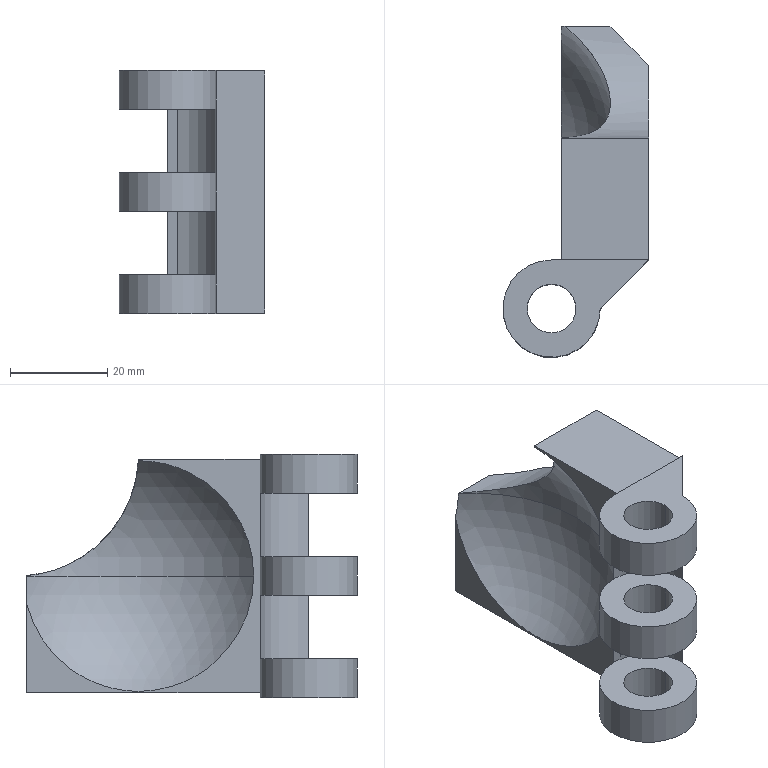Part | SolidWorks | features BaseBody 1 | 1 solid | 28 faces | box 30 x 68 x 50 mm | volume 32451 mm3 | plane 14 | cylinder 12 | sphere 2 | commonest cylinder face diameters 10 x6 20 x5 50 x1
STEP:
#1=CARTESIAN_POINT('',(-5.,0.,29.));
#2=VERTEX_POINT('',#1);
#3=CARTESIAN_POINT('',(5.,0.,29.));
#4=VERTEX_POINT('',#3);
#5=CARTESIAN_POINT('',(0.,0.,29.));
#6=DIRECTION('',(0.,0.,1.));
#7=DIRECTION('',(-1.,0.,0.));
#8=AXIS2_PLACEMENT_3D('',#5,#6,#7);
#9=CIRCLE('',#8,5.);
#10=EDGE_CURVE('',#2,#4,#9,.T.);
#11=ORIENTED_EDGE('',*,*,#10,.T.);
#12=CARTESIAN_POINT('',(5.,0.,21.));
#13=VERTEX_POINT('',#12);
#14=CARTESIAN_POINT('',(5.,0.,0.));
#15=DIRECTION('',(0.,0.,-1.));
#16=VECTOR('',#15,1000.);
#17=LINE('',#14,#16);
#18=EDGE_CURVE('',#4,#13,#17,.T.);
#19=ORIENTED_EDGE('',*,*,#18,.T.);
#20=CARTESIAN_POINT('',(-5.,0.,21.));
#21=VERTEX_POINT('',#20);
#22=CARTESIAN_POINT('',(0.,0.,21.));
#23=DIRECTION('',(0.,0.,-1.));
#24=DIRECTION('',(-1.,0.,0.));
#25=AXIS2_PLACEMENT_3D('',#22,#23,#24);
#26=CIRCLE('',#25,5.);
#27=EDGE_CURVE('',#13,#21,#26,.T.);
#28=ORIENTED_EDGE('',*,*,#27,.T.);
#29=CARTESIAN_POINT('',(-5.,0.,0.));
#30=DIRECTION('',(0.,0.,-1.));
#31=VECTOR('',#30,1000.);
#32=LINE('',#29,#31);
#33=EDGE_CURVE('',#2,#21,#32,.T.);
#34=ORIENTED_EDGE('',*,*,#33,.F.);
#35=EDGE_LOOP('',(#11,#19,#28,#34));
#36=FACE_OUTER_BOUND('',#35,.T.);
#37=CARTESIAN_POINT('',(0.,0.,0.));
#38=DIRECTION('',(0.,0.,-1.));
#39=DIRECTION('',(-1.,0.,0.));
#40=AXIS2_PLACEMENT_3D('',#37,#38,#39);
#41=CYLINDRICAL_SURFACE('',#40,5.);
#42=ADVANCED_FACE('',(#36),#41,.F.);
#43=CARTESIAN_POINT('',(5.,0.,50.));
#44=VERTEX_POINT('',#43);
#45=CARTESIAN_POINT('',(-5.,0.,50.));
#46=VERTEX_POINT('',#45);
#47=CARTESIAN_POINT('',(0.,0.,50.));
#48=DIRECTION('',(0.,0.,-1.));
#49=DIRECTION('',(-1.,0.,0.));
#50=AXIS2_PLACEMENT_3D('',#47,#48,#49);
#51=CIRCLE('',#50,5.);
#52=EDGE_CURVE('',#44,#46,#51,.T.);
#53=ORIENTED_EDGE('',*,*,#52,.F.);
#54=CARTESIAN_POINT('',(5.,0.,42.));
#55=VERTEX_POINT('',#54);
#56=CARTESIAN_POINT('',(5.,0.,0.));
#57=DIRECTION('',(0.,0.,-1.));
#58=VECTOR('',#57,1000.);
#59=LINE('',#56,#58);
#60=EDGE_CURVE('',#44,#55,#59,.T.);
#61=ORIENTED_EDGE('',*,*,#60,.T.);
#62=CARTESIAN_POINT('',(-5.,0.,42.));
#63=VERTEX_POINT('',#62);
#64=CARTESIAN_POINT('',(0.,0.,42.));
#65=DIRECTION('',(0.,0.,-1.));
#66=DIRECTION('',(-1.,0.,0.));
#67=AXIS2_PLACEMENT_3D('',#64,#65,#66);
#68=CIRCLE('',#67,5.);
#69=EDGE_CURVE('',#55,#63,#68,.T.);
#70=ORIENTED_EDGE('',*,*,#69,.T.);
#71=CARTESIAN_POINT('',(-5.,0.,0.));
#72=DIRECTION('',(0.,0.,-1.));
#73=VECTOR('',#72,1000.);
#74=LINE('',#71,#73);
#75=EDGE_CURVE('',#46,#63,#74,.T.);
#76=ORIENTED_EDGE('',*,*,#75,.F.);
#77=EDGE_LOOP('',(#53,#61,#70,#76));
#78=FACE_OUTER_BOUND('',#77,.T.);
#79=CARTESIAN_POINT('',(0.,0.,0.));
#80=DIRECTION('',(0.,0.,-1.));
#81=DIRECTION('',(-1.,0.,0.));
#82=AXIS2_PLACEMENT_3D('',#79,#80,#81);
#83=CYLINDRICAL_SURFACE('',#82,5.);
#84=ADVANCED_FACE('',(#78),#83,.F.);
#85=CARTESIAN_POINT('',(2.,58.,19.458));
#86=VERTEX_POINT('',#85);
#87=CARTESIAN_POINT('',(2.,11.342,25.));
#88=VERTEX_POINT('',#87);
#89=CARTESIAN_POINT('',(2.,35.,25.));
#90=DIRECTION('',(-1.,0.,0.));
#91=DIRECTION('',(0.,0.,1.));
#92=AXIS2_PLACEMENT_3D('',#89,#90,#91);
#93=CIRCLE('',#92,23.658);
#94=EDGE_CURVE('',#86,#88,#93,.T.);
#95=ORIENTED_EDGE('',*,*,#94,.T.);
#96=CARTESIAN_POINT('',(2.865,58.,25.));
#97=VERTEX_POINT('',#96);
#98=CARTESIAN_POINT('',(-15.321,35.,25.));
#99=DIRECTION('',(0.,0.,1.));
#100=DIRECTION('',(1.,0.,0.));
#101=AXIS2_PLACEMENT_3D('',#98,#99,#100);
#102=CIRCLE('',#101,29.321);
#103=EDGE_CURVE('',#88,#97,#102,.T.);
#104=ORIENTED_EDGE('',*,*,#103,.T.);
#105=CARTESIAN_POINT('',(-15.321,58.,25.));
#106=DIRECTION('',(0.,1.,0.));
#107=DIRECTION('',(0.,0.,1.));
#108=AXIS2_PLACEMENT_3D('',#105,#106,#107);
#109=CIRCLE('',#108,18.186);
#110=EDGE_CURVE('',#97,#86,#109,.T.);
#111=ORIENTED_EDGE('',*,*,#110,.T.);
#112=EDGE_LOOP('',(#95,#104,#111));
#113=FACE_OUTER_BOUND('',#112,.T.);
#114=CARTESIAN_POINT('',(-15.321,35.,25.));
#115=DIRECTION('',(0.,0.,-1.));
#116=DIRECTION('',(1.,0.,0.));
#117=AXIS2_PLACEMENT_3D('',#114,#115,#116);
#118=SPHERICAL_SURFACE('',#117,29.321);
#119=ADVANCED_FACE('',(#113),#118,.F.);
#120=CARTESIAN_POINT('',(-5.,0.,8.));
#121=VERTEX_POINT('',#120);
#122=CARTESIAN_POINT('',(5.,0.,8.));
#123=VERTEX_POINT('',#122);
#124=CARTESIAN_POINT('',(0.,0.,8.));
#125=DIRECTION('',(0.,0.,1.));
#126=DIRECTION('',(-1.,0.,0.));
#127=AXIS2_PLACEMENT_3D('',#124,#125,#126);
#128=CIRCLE('',#127,5.);
#129=EDGE_CURVE('',#121,#123,#128,.T.);
#130=ORIENTED_EDGE('',*,*,#129,.T.);
#131=CARTESIAN_POINT('',(5.,0.,0.));
#132=VERTEX_POINT('',#131);
#133=CARTESIAN_POINT('',(5.,0.,0.));
#134=DIRECTION('',(0.,0.,-1.));
#135=VECTOR('',#134,1000.);
#136=LINE('',#133,#135);
#137=EDGE_CURVE('',#123,#132,#136,.T.);
#138=ORIENTED_EDGE('',*,*,#137,.T.);
#139=CARTESIAN_POINT('',(-5.,0.,0.));
#140=VERTEX_POINT('',#139);
#141=CARTESIAN_POINT('',(0.,0.,0.));
#142=DIRECTION('',(0.,0.,1.));
#143=DIRECTION('',(-1.,0.,0.));
#144=AXIS2_PLACEMENT_3D('',#141,#142,#143);
#145=CIRCLE('',#144,5.);
#146=EDGE_CURVE('',#140,#132,#145,.T.);
#147=ORIENTED_EDGE('',*,*,#146,.F.);
#148=CARTESIAN_POINT('',(-5.,0.,0.));
#149=DIRECTION('',(0.,0.,-1.));
#150=VECTOR('',#149,1000.);
#151=LINE('',#148,#150);
#152=EDGE_CURVE('',#121,#140,#151,.T.);
#153=ORIENTED_EDGE('',*,*,#152,.F.);
#154=EDGE_LOOP('',(#130,#138,#147,#153));
#155=FACE_OUTER_BOUND('',#154,.T.);
#156=CARTESIAN_POINT('',(0.,0.,0.));
#157=DIRECTION('',(0.,0.,-1.));
#158=DIRECTION('',(-1.,0.,0.));
#159=AXIS2_PLACEMENT_3D('',#156,#157,#158);
#160=CYLINDRICAL_SURFACE('',#159,5.);
#161=ADVANCED_FACE('',(#155),#160,.F.);
#162=ORIENTED_EDGE('',*,*,#10,.F.);
#163=CARTESIAN_POINT('',(0.,0.,29.));
#164=DIRECTION('',(0.,0.,1.));
#165=DIRECTION('',(-1.,0.,0.));
#166=AXIS2_PLACEMENT_3D('',#163,#164,#165);
#167=CIRCLE('',#166,5.);
#168=EDGE_CURVE('',#4,#2,#167,.T.);
#169=ORIENTED_EDGE('',*,*,#168,.F.);
#170=EDGE_LOOP('',(#162,#169));
#171=FACE_BOUND('',#170,.T.);
#172=CARTESIAN_POINT('',(10.,0.,29.));
#173=VERTEX_POINT('',#172);
#174=CARTESIAN_POINT('',(0.,10.,29.));
#175=VERTEX_POINT('',#174);
#176=CARTESIAN_POINT('',(0.,0.,29.));
#177=DIRECTION('',(0.,0.,-1.));
#178=DIRECTION('',(0.,1.,0.));
#179=AXIS2_PLACEMENT_3D('',#176,#177,#178);
#180=CIRCLE('',#179,10.);
#181=EDGE_CURVE('',#173,#175,#180,.T.);
#182=ORIENTED_EDGE('',*,*,#181,.F.);
#183=CARTESIAN_POINT('',(0.,0.,29.));
#184=DIRECTION('',(0.,0.,-1.));
#185=DIRECTION('',(1.,0.,0.));
#186=AXIS2_PLACEMENT_3D('',#183,#184,#185);
#187=CIRCLE('',#186,10.);
#188=EDGE_CURVE('',#175,#173,#187,.T.);
#189=ORIENTED_EDGE('',*,*,#188,.F.);
#190=EDGE_LOOP('',(#182,#189));
#191=FACE_OUTER_BOUND('',#190,.T.);
#192=CARTESIAN_POINT('',(0.,0.,29.));
#193=DIRECTION('',(0.,0.,-1.));
#194=DIRECTION('',(0.,-1.,0.));
#195=AXIS2_PLACEMENT_3D('',#192,#193,#194);
#196=PLANE('',#195);
#197=ADVANCED_FACE('',(#171,#191),#196,.F.);
#198=CARTESIAN_POINT('',(0.,0.,42.));
#199=DIRECTION('',(0.,0.,-1.));
#200=DIRECTION('',(-1.,0.,0.));
#201=AXIS2_PLACEMENT_3D('',#198,#199,#200);
#202=CIRCLE('',#201,5.);
#203=EDGE_CURVE('',#63,#55,#202,.T.);
#204=ORIENTED_EDGE('',*,*,#203,.F.);
#205=ORIENTED_EDGE('',*,*,#69,.F.);
#206=EDGE_LOOP('',(#204,#205));
#207=FACE_BOUND('',#206,.T.);
#208=CARTESIAN_POINT('',(0.,10.,42.));
#209=VERTEX_POINT('',#208);
#210=CARTESIAN_POINT('',(10.,0.,42.));
#211=VERTEX_POINT('',#210);
#212=CARTESIAN_POINT('',(0.,0.,42.));
#213=DIRECTION('',(0.,0.,1.));
#214=DIRECTION('',(0.,1.,0.));
#215=AXIS2_PLACEMENT_3D('',#212,#213,#214);
#216=CIRCLE('',#215,10.);
#217=EDGE_CURVE('',#209,#211,#216,.T.);
#218=ORIENTED_EDGE('',*,*,#217,.F.);
#219=CARTESIAN_POINT('',(0.,0.,42.));
#220=DIRECTION('',(0.,0.,-1.));
#221=DIRECTION('',(1.,0.,0.));
#222=AXIS2_PLACEMENT_3D('',#219,#220,#221);
#223=CIRCLE('',#222,10.);
#224=EDGE_CURVE('',#209,#211,#223,.T.);
#225=ORIENTED_EDGE('',*,*,#224,.T.);
#226=EDGE_LOOP('',(#218,#225));
#227=FACE_OUTER_BOUND('',#226,.T.);
#228=CARTESIAN_POINT('',(-10.,0.,42.));
#229=DIRECTION('',(0.,0.,1.));
#230=DIRECTION('',(1.,0.,0.));
#231=AXIS2_PLACEMENT_3D('',#228,#229,#230);
#232=PLANE('',#231);
#233=ADVANCED_FACE('',(#207,#227),#232,.F.);
#234=CARTESIAN_POINT('',(10.,0.,0.));
#235=DIRECTION('',(0.,0.,1.));
#236=VECTOR('',#235,1000.);
#237=LINE('',#234,#236);
#238=EDGE_CURVE('',#173,#211,#237,.T.);
#239=ORIENTED_EDGE('',*,*,#238,.T.);
#240=ORIENTED_EDGE('',*,*,#224,.F.);
#241=CARTESIAN_POINT('',(0.,10.,0.));
#242=DIRECTION('',(0.,0.,1.));
#243=VECTOR('',#242,1000.);
#244=LINE('',#241,#243);
#245=EDGE_CURVE('',#175,#209,#244,.T.);
#246=ORIENTED_EDGE('',*,*,#245,.F.);
#247=ORIENTED_EDGE('',*,*,#188,.T.);
#248=EDGE_LOOP('',(#239,#240,#246,#247));
#249=FACE_OUTER_BOUND('',#248,.T.);
#250=CARTESIAN_POINT('',(0.,0.,35.5));
#251=DIRECTION('',(0.,0.,1.));
#252=DIRECTION('',(-1.,0.,0.));
#253=AXIS2_PLACEMENT_3D('',#250,#251,#252);
#254=CYLINDRICAL_SURFACE('',#253,10.);
#255=ADVANCED_FACE('',(#249),#254,.F.);
#256=CARTESIAN_POINT('',(0.,10.,8.));
#257=VERTEX_POINT('',#256);
#258=CARTESIAN_POINT('',(0.,10.,21.));
#259=VERTEX_POINT('',#258);
#260=CARTESIAN_POINT('',(0.,10.,0.));
#261=DIRECTION('',(0.,0.,1.));
#262=VECTOR('',#261,1000.);
#263=LINE('',#260,#262);
#264=EDGE_CURVE('',#257,#259,#263,.T.);
#265=ORIENTED_EDGE('',*,*,#264,.F.);
#266=CARTESIAN_POINT('',(10.,0.,8.));
#267=VERTEX_POINT('',#266);
#268=CARTESIAN_POINT('',(0.,0.,8.));
#269=DIRECTION('',(0.,0.,-1.));
#270=DIRECTION('',(1.,0.,0.));
#271=AXIS2_PLACEMENT_3D('',#268,#269,#270);
#272=CIRCLE('',#271,10.);
#273=EDGE_CURVE('',#257,#267,#272,.T.);
#274=ORIENTED_EDGE('',*,*,#273,.T.);
#275=CARTESIAN_POINT('',(10.,0.,21.));
#276=VERTEX_POINT('',#275);
#277=CARTESIAN_POINT('',(10.,0.,0.));
#278=DIRECTION('',(0.,0.,1.));
#279=VECTOR('',#278,1000.);
#280=LINE('',#277,#279);
#281=EDGE_CURVE('',#267,#276,#280,.T.);
#282=ORIENTED_EDGE('',*,*,#281,.T.);
#283=CARTESIAN_POINT('',(0.,0.,21.));
#284=DIRECTION('',(0.,0.,-1.));
#285=DIRECTION('',(1.,0.,0.));
#286=AXIS2_PLACEMENT_3D('',#283,#284,#285);
#287=CIRCLE('',#286,10.);
#288=EDGE_CURVE('',#259,#276,#287,.T.);
#289=ORIENTED_EDGE('',*,*,#288,.F.);
#290=EDGE_LOOP('',(#265,#274,#282,#289));
#291=FACE_OUTER_BOUND('',#290,.T.);
#292=CARTESIAN_POINT('',(0.,0.,14.5));
#293=DIRECTION('',(0.,0.,1.));
#294=DIRECTION('',(-1.,0.,0.));
#295=AXIS2_PLACEMENT_3D('',#292,#293,#294);
#296=CYLINDRICAL_SURFACE('',#295,10.);
#297=ADVANCED_FACE('',(#291),#296,.F.);
#298=ORIENTED_EDGE('',*,*,#129,.F.);
#299=CARTESIAN_POINT('',(0.,0.,8.));
#300=DIRECTION('',(0.,0.,1.));
#301=DIRECTION('',(-1.,0.,0.));
#302=AXIS2_PLACEMENT_3D('',#299,#300,#301);
#303=CIRCLE('',#302,5.);
#304=EDGE_CURVE('',#123,#121,#303,.T.);
#305=ORIENTED_EDGE('',*,*,#304,.F.);
#306=EDGE_LOOP('',(#298,#305));
#307=FACE_BOUND('',#306,.T.);
#308=CARTESIAN_POINT('',(0.,0.,8.));
#309=DIRECTION('',(0.,0.,-1.));
#310=DIRECTION('',(0.,1.,0.));
#311=AXIS2_PLACEMENT_3D('',#308,#309,#310);
#312=CIRCLE('',#311,10.);
#313=EDGE_CURVE('',#267,#257,#312,.T.);
#314=ORIENTED_EDGE('',*,*,#313,.F.);
#315=ORIENTED_EDGE('',*,*,#273,.F.);
#316=EDGE_LOOP('',(#314,#315));
#317=FACE_OUTER_BOUND('',#316,.T.);
#318=CARTESIAN_POINT('',(0.,0.,8.));
#319=DIRECTION('',(0.,0.,-1.));
#320=DIRECTION('',(0.,-1.,0.));
#321=AXIS2_PLACEMENT_3D('',#318,#319,#320);
#322=PLANE('',#321);
#323=ADVANCED_FACE('',(#307,#317),#322,.F.);
#324=CARTESIAN_POINT('',(0.,0.,21.));
#325=DIRECTION('',(0.,0.,-1.));
#326=DIRECTION('',(-1.,0.,0.));
#327=AXIS2_PLACEMENT_3D('',#324,#325,#326);
#328=CIRCLE('',#327,5.);
#329=EDGE_CURVE('',#21,#13,#328,.T.);
#330=ORIENTED_EDGE('',*,*,#329,.F.);
#331=ORIENTED_EDGE('',*,*,#27,.F.);
#332=EDGE_LOOP('',(#330,#331));
#333=FACE_BOUND('',#332,.T.);
#334=CARTESIAN_POINT('',(0.,0.,21.));
#335=DIRECTION('',(0.,0.,1.));
#336=DIRECTION('',(0.,1.,0.));
#337=AXIS2_PLACEMENT_3D('',#334,#335,#336);
#338=CIRCLE('',#337,10.);
#339=EDGE_CURVE('',#259,#276,#338,.T.);
#340=ORIENTED_EDGE('',*,*,#339,.F.);
#341=ORIENTED_EDGE('',*,*,#288,.T.);
#342=EDGE_LOOP('',(#340,#341));
#343=FACE_OUTER_BOUND('',#342,.T.);
#344=CARTESIAN_POINT('',(-10.,0.,21.));
#345=DIRECTION('',(0.,0.,1.));
#346=DIRECTION('',(1.,0.,0.));
#347=AXIS2_PLACEMENT_3D('',#344,#345,#346);
#348=PLANE('',#347);
#349=ADVANCED_FACE('',(#333,#343),#348,.F.);
#350=ORIENTED_EDGE('',*,*,#313,.T.);
#351=CARTESIAN_POINT('',(0.,10.,0.));
#352=VERTEX_POINT('',#351);
#353=CARTESIAN_POINT('',(0.,10.,0.));
#354=DIRECTION('',(0.,0.,1.));
#355=VECTOR('',#354,1000.);
#356=LINE('',#353,#355);
#357=EDGE_CURVE('',#352,#257,#356,.T.);
#358=ORIENTED_EDGE('',*,*,#357,.F.);
#359=CARTESIAN_POINT('',(10.,0.,0.));
#360=VERTEX_POINT('',#359);
#361=CARTESIAN_POINT('',(0.,0.,0.));
#362=DIRECTION('',(0.,0.,1.));
#363=DIRECTION('',(0.,1.,0.));
#364=AXIS2_PLACEMENT_3D('',#361,#362,#363);
#365=CIRCLE('',#364,10.);
#366=EDGE_CURVE('',#352,#360,#365,.T.);
#367=ORIENTED_EDGE('',*,*,#366,.T.);
#368=CARTESIAN_POINT('',(10.,0.,0.));
#369=DIRECTION('',(0.,0.,1.));
#370=VECTOR('',#369,1000.);
#371=LINE('',#368,#370);
#372=EDGE_CURVE('',#360,#267,#371,.T.);
#373=ORIENTED_EDGE('',*,*,#372,.T.);
#374=EDGE_LOOP('',(#350,#358,#367,#373));
#375=FACE_OUTER_BOUND('',#374,.T.);
#376=CARTESIAN_POINT('',(0.,0.,0.));
#377=DIRECTION('',(0.,0.,-1.));
#378=DIRECTION('',(0.,1.,0.));
#379=AXIS2_PLACEMENT_3D('',#376,#377,#378);
#380=CYLINDRICAL_SURFACE('',#379,10.);
#381=ADVANCED_FACE('',(#375),#380,.T.);
#382=ORIENTED_EDGE('',*,*,#217,.T.);
#383=CARTESIAN_POINT('',(10.,0.,50.));
#384=VERTEX_POINT('',#383);
#385=CARTESIAN_POINT('',(10.,0.,0.));
#386=DIRECTION('',(0.,0.,1.));
#387=VECTOR('',#386,1000.);
#388=LINE('',#385,#387);
#389=EDGE_CURVE('',#211,#384,#388,.T.);
#390=ORIENTED_EDGE('',*,*,#389,.T.);
#391=CARTESIAN_POINT('',(0.,10.,50.));
#392=VERTEX_POINT('',#391);
#393=CARTESIAN_POINT('',(0.,0.,50.));
#394=DIRECTION('',(0.,0.,1.));
#395=DIRECTION('',(0.,1.,0.));
#396=AXIS2_PLACEMENT_3D('',#393,#394,#395);
#397=CIRCLE('',#396,10.);
#398=EDGE_CURVE('',#392,#384,#397,.T.);
#399=ORIENTED_EDGE('',*,*,#398,.F.);
#400=CARTESIAN_POINT('',(0.,10.,0.));
#401=DIRECTION('',(0.,0.,1.));
#402=VECTOR('',#401,1000.);
#403=LINE('',#400,#402);
#404=EDGE_CURVE('',#209,#392,#403,.T.);
#405=ORIENTED_EDGE('',*,*,#404,.F.);
#406=EDGE_LOOP('',(#382,#390,#399,#405));
#407=FACE_OUTER_BOUND('',#406,.T.);
#408=CARTESIAN_POINT('',(0.,0.,0.));
#409=DIRECTION('',(0.,0.,-1.));
#410=DIRECTION('',(0.,1.,0.));
#411=AXIS2_PLACEMENT_3D('',#408,#409,#410);
#412=CYLINDRICAL_SURFACE('',#411,10.);
#413=ADVANCED_FACE('',(#407),#412,.T.);
#414=ORIENTED_EDGE('',*,*,#181,.T.);
#415=CARTESIAN_POINT('',(0.,10.,0.));
#416=DIRECTION('',(0.,0.,1.));
#417=VECTOR('',#416,1000.);
#418=LINE('',#415,#417);
#419=EDGE_CURVE('',#259,#175,#418,.T.);
#420=ORIENTED_EDGE('',*,*,#419,.F.);
#421=ORIENTED_EDGE('',*,*,#339,.T.);
#422=CARTESIAN_POINT('',(10.,0.,0.));
#423=DIRECTION('',(0.,0.,1.));
#424=VECTOR('',#423,1000.);
#425=LINE('',#422,#424);
#426=EDGE_CURVE('',#276,#173,#425,.T.);
#427=ORIENTED_EDGE('',*,*,#426,.T.);
#428=EDGE_LOOP('',(#414,#420,#421,#427));
#429=FACE_OUTER_BOUND('',#428,.T.);
#430=CARTESIAN_POINT('',(0.,0.,0.));
#431=DIRECTION('',(0.,0.,-1.));
#432=DIRECTION('',(0.,1.,0.));
#433=AXIS2_PLACEMENT_3D('',#430,#431,#432);
#434=CYLINDRICAL_SURFACE('',#433,10.);
#435=ADVANCED_FACE('',(#429),#434,.T.);
#436=CARTESIAN_POINT('',(12.,58.,25.08));
#437=VERTEX_POINT('',#436);
#438=CARTESIAN_POINT('',(20.,50.,27.087));
#439=VERTEX_POINT('',#438);
#440=CARTESIAN_POINT('',(12.,58.,25.08));
#441=CARTESIAN_POINT('',(14.766,55.234,25.302));
#442=CARTESIAN_POINT('',(17.457,52.543,25.977));
#443=CARTESIAN_POINT('',(20.,50.,27.087));
#444=(BOUNDED_CURVE()B_SPLINE_CURVE(3,(#440,#441,#442,#443),.UNSPECIFIED.,.F.,.T.)B_SPLINE_CURVE_WITH_KNOTS((4,4),(1.651,1.982),.UNSPECIFIED.)CURVE()GEOMETRIC_REPRESENTATION_ITEM()RATIONAL_B_SPLINE_CURVE((1.,0.9909,0.9909,1.))REPRESENTATION_ITEM(''));
#445=EDGE_CURVE('',#437,#439,#444,.T.);
#446=ORIENTED_EDGE('',*,*,#445,.F.);
#447=CARTESIAN_POINT('',(2.865,58.,25.08));
#448=VERTEX_POINT('',#447);
#449=CARTESIAN_POINT('',(20.,58.,25.08));
#450=DIRECTION('',(1.,0.,0.));
#451=VECTOR('',#450,1000.);
#452=LINE('',#449,#451);
#453=EDGE_CURVE('',#448,#437,#452,.T.);
#454=ORIENTED_EDGE('',*,*,#453,.F.);
#455=CARTESIAN_POINT('',(2.,35.036,48.658));
#456=VERTEX_POINT('',#455);
#457=CARTESIAN_POINT('',(2.,35.036,48.658));
#458=CARTESIAN_POINT('',(3.428,35.092,47.612));
#459=CARTESIAN_POINT('',(4.74,35.219,46.455));
#460=CARTESIAN_POINT('',(6.232,35.528,44.877));
#461=CARTESIAN_POINT('',(6.524,35.598,44.555));
#462=CARTESIAN_POINT('',(7.09,35.754,43.897));
#463=CARTESIAN_POINT('',(7.367,35.841,43.56));
#464=CARTESIAN_POINT('',(8.164,36.128,42.541));
#465=CARTESIAN_POINT('',(8.653,36.354,41.85));
#466=CARTESIAN_POINT('',(9.544,36.884,40.449));
#467=CARTESIAN_POINT('',(9.947,37.189,39.738));
#468=CARTESIAN_POINT('',(10.484,37.716,38.661));
#469=CARTESIAN_POINT('',(10.652,37.903,38.3));
#470=CARTESIAN_POINT('',(10.964,38.303,37.574));
#471=CARTESIAN_POINT('',(11.108,38.516,37.209));
#472=CARTESIAN_POINT('',(11.495,39.182,36.132));
#473=CARTESIAN_POINT('',(11.697,39.668,35.428));
#474=CARTESIAN_POINT('',(11.915,40.462,34.398));
#475=CARTESIAN_POINT('',(11.973,40.737,34.058));
#476=CARTESIAN_POINT('',(12.06,41.311,33.389));
#477=CARTESIAN_POINT('',(12.089,41.611,33.058));
#478=CARTESIAN_POINT('',(12.128,42.525,32.1));
#479=CARTESIAN_POINT('',(12.095,43.164,31.499));
#480=CARTESIAN_POINT('',(11.956,44.163,30.651));
#481=CARTESIAN_POINT('',(11.895,44.503,30.378));
#482=CARTESIAN_POINT('',(11.742,45.197,29.849));
#483=CARTESIAN_POINT('',(11.651,45.552,29.593));
#484=CARTESIAN_POINT('',(11.336,46.617,28.867));
#485=CARTESIAN_POINT('',(11.072,47.334,28.431));
#486=CARTESIAN_POINT('',(10.599,48.417,27.842));
#487=CARTESIAN_POINT('',(10.428,48.779,27.656));
#488=CARTESIAN_POINT('',(10.06,49.505,27.306));
#489=CARTESIAN_POINT('',(9.863,49.87,27.141));
#490=CARTESIAN_POINT('',(9.242,50.948,26.683));
#491=CARTESIAN_POINT('',(8.785,51.655,26.423));
#492=CARTESIAN_POINT('',(8.039,52.693,26.089));
#493=CARTESIAN_POINT('',(7.781,53.035,25.987));
#494=CARTESIAN_POINT('',(7.243,53.712,25.801));
#495=CARTESIAN_POINT('',(6.963,54.048,25.717));
#496=CARTESIAN_POINT('',(5.527,55.691,25.337));
#497=CARTESIAN_POINT('',(4.255,56.9,25.168));
#498=CARTESIAN_POINT('',(2.865,58.,25.08));
#499=B_SPLINE_CURVE_WITH_KNOTS('',3,(#457,#458,#459,#460,#461,#462,#463,#464,#465,#466,#467,#468,#469,#470,#471,#472,#473,#474,#475,#476,#477,#478,#479,#480,#481,#482,#483,#484,#485,#486,#487,#488,#489,#490,#491,#492,#493,#494,#495,#496,#497,#498),.UNSPECIFIED.,.F.,.F.,(4,2,2,2,2,2,2,2,2,2,2,2,2,2,2,2,2,2,2,2,4),(0.,0.005255,0.006569,0.007883,0.01051,0.01314,0.01445,0.01577,0.01839,0.01971,0.02102,0.02365,0.02496,0.02628,0.0289,0.03022,0.03153,0.03416,0.03547,0.03679,0.04204),.UNSPECIFIED.);
#500=EDGE_CURVE('',#456,#448,#499,.T.);
#501=ORIENTED_EDGE('',*,*,#500,.F.);
#502=CARTESIAN_POINT('',(2.,35.02,49.));
#503=VERTEX_POINT('',#502);
#504=CARTESIAN_POINT('',(2.,60.,50.));
#505=DIRECTION('',(1.,0.,0.));
#506=DIRECTION('',(0.,0.,1.));
#507=AXIS2_PLACEMENT_3D('',#504,#505,#506);
#508=CIRCLE('',#507,25.);
#509=EDGE_CURVE('',#503,#456,#508,.T.);
#510=ORIENTED_EDGE('',*,*,#509,.F.);
#511=CARTESIAN_POINT('',(20.,35.02,49.));
#512=VERTEX_POINT('',#511);
#513=CARTESIAN_POINT('',(20.,35.02,49.));
#514=DIRECTION('',(-1.,0.,0.));
#515=VECTOR('',#514,1000.);
#516=LINE('',#513,#515);
#517=EDGE_CURVE('',#512,#503,#516,.T.);
#518=ORIENTED_EDGE('',*,*,#517,.F.);
#519=CARTESIAN_POINT('',(20.,60.,50.));
#520=DIRECTION('',(-1.,0.,0.));
#521=DIRECTION('',(0.,0.,1.));
#522=AXIS2_PLACEMENT_3D('',#519,#520,#521);
#523=CIRCLE('',#522,25.);
#524=EDGE_CURVE('',#439,#512,#523,.T.);
#525=ORIENTED_EDGE('',*,*,#524,.F.);
#526=EDGE_LOOP('',(#446,#454,#501,#510,#518,#525));
#527=FACE_OUTER_BOUND('',#526,.T.);
#528=CARTESIAN_POINT('',(20.,60.,50.));
#529=DIRECTION('',(1.,0.,0.));
#530=DIRECTION('',(0.,0.,1.));
#531=AXIS2_PLACEMENT_3D('',#528,#529,#530);
#532=CYLINDRICAL_SURFACE('',#531,25.);
#533=ADVANCED_FACE('',(#527),#532,.F.);
#534=ORIENTED_EDGE('',*,*,#453,.T.);
#535=CARTESIAN_POINT('',(12.,58.,1.));
#536=VERTEX_POINT('',#535);
#537=CARTESIAN_POINT('',(12.,58.,25.));
#538=DIRECTION('',(0.,0.,1.));
#539=VECTOR('',#538,1000.);
#540=LINE('',#537,#539);
#541=EDGE_CURVE('',#536,#437,#540,.T.);
#542=ORIENTED_EDGE('',*,*,#541,.F.);
#543=CARTESIAN_POINT('',(2.,58.,1.));
#544=VERTEX_POINT('',#543);
#545=CARTESIAN_POINT('',(16.,58.,1.));
#546=DIRECTION('',(-1.,0.,0.));
#547=VECTOR('',#546,1000.);
#548=LINE('',#545,#547);
#549=EDGE_CURVE('',#536,#544,#548,.T.);
#550=ORIENTED_EDGE('',*,*,#549,.T.);
#551=CARTESIAN_POINT('',(2.,58.,50.));
#552=DIRECTION('',(0.,0.,-1.));
#553=VECTOR('',#552,1000.);
#554=LINE('',#551,#553);
#555=EDGE_CURVE('',#86,#544,#554,.T.);
#556=ORIENTED_EDGE('',*,*,#555,.F.);
#557=ORIENTED_EDGE('',*,*,#110,.F.);
#558=CARTESIAN_POINT('',(-15.321,58.,25.));
#559=DIRECTION('',(0.,1.,0.));
#560=DIRECTION('',(0.,0.,1.));
#561=AXIS2_PLACEMENT_3D('',#558,#559,#560);
#562=CIRCLE('',#561,18.186);
#563=EDGE_CURVE('',#448,#97,#562,.T.);
#564=ORIENTED_EDGE('',*,*,#563,.F.);
#565=EDGE_LOOP('',(#534,#542,#550,#556,#557,#564));
#566=FACE_OUTER_BOUND('',#565,.T.);
#567=CARTESIAN_POINT('',(12.,58.,50.));
#568=DIRECTION('',(0.,-1.,0.));
#569=DIRECTION('',(0.,0.,-1.));
#570=AXIS2_PLACEMENT_3D('',#567,#568,#569);
#571=PLANE('',#570);
#572=ADVANCED_FACE('',(#566),#571,.F.);
#573=ORIENTED_EDGE('',*,*,#445,.T.);
#574=CARTESIAN_POINT('',(20.,50.,1.));
#575=VERTEX_POINT('',#574);
#576=CARTESIAN_POINT('',(20.,50.,0.));
#577=DIRECTION('',(0.,0.,1.));
#578=VECTOR('',#577,1000.);
#579=LINE('',#576,#578);
#580=EDGE_CURVE('',#575,#439,#579,.T.);
#581=ORIENTED_EDGE('',*,*,#580,.F.);
#582=CARTESIAN_POINT('',(18.,52.,1.));
#583=DIRECTION('',(-0.7071,0.7071,0.));
#584=VECTOR('',#583,1000.);
#585=LINE('',#582,#584);
#586=EDGE_CURVE('',#575,#536,#585,.T.);
#587=ORIENTED_EDGE('',*,*,#586,.T.);
#588=ORIENTED_EDGE('',*,*,#541,.T.);
#589=EDGE_LOOP('',(#573,#581,#587,#588));
#590=FACE_OUTER_BOUND('',#589,.T.);
#591=CARTESIAN_POINT('',(20.,50.,0.));
#592=DIRECTION('',(0.7071,0.7071,0.));
#593=DIRECTION('',(0.,0.,-1.));
#594=AXIS2_PLACEMENT_3D('',#591,#592,#593);
#595=PLANE('',#594);
#596=ADVANCED_FACE('',(#590),#595,.T.);
#597=ORIENTED_EDGE('',*,*,#524,.T.);
#598=CARTESIAN_POINT('',(20.,10.,49.));
#599=VERTEX_POINT('',#598);
#600=CARTESIAN_POINT('',(20.,34.,49.));
#601=DIRECTION('',(0.,-1.,0.));
#602=VECTOR('',#601,1000.);
#603=LINE('',#600,#602);
#604=EDGE_CURVE('',#512,#599,#603,.T.);
#605=ORIENTED_EDGE('',*,*,#604,.T.);
#606=CARTESIAN_POINT('',(20.,10.,1.));
#607=VERTEX_POINT('',#606);
#608=CARTESIAN_POINT('',(20.,10.,0.));
#609=DIRECTION('',(0.,0.,1.));
#610=VECTOR('',#609,1000.);
#611=LINE('',#608,#610);
#612=EDGE_CURVE('',#607,#599,#611,.T.);
#613=ORIENTED_EDGE('',*,*,#612,.F.);
#614=CARTESIAN_POINT('',(20.,34.,1.));
#615=DIRECTION('',(0.,1.,0.));
#616=VECTOR('',#615,1000.);
#617=LINE('',#614,#616);
#618=EDGE_CURVE('',#607,#575,#617,.T.);
#619=ORIENTED_EDGE('',*,*,#618,.T.);
#620=ORIENTED_EDGE('',*,*,#580,.T.);
#621=EDGE_LOOP('',(#597,#605,#613,#619,#620));
#622=FACE_OUTER_BOUND('',#621,.T.);
#623=CARTESIAN_POINT('',(20.,10.,0.));
#624=DIRECTION('',(1.,0.,0.));
#625=DIRECTION('',(0.,1.,0.));
#626=AXIS2_PLACEMENT_3D('',#623,#624,#625);
#627=PLANE('',#626);
#628=ADVANCED_FACE('',(#622),#627,.T.);
#629=ORIENTED_EDGE('',*,*,#586,.F.);
#630=ORIENTED_EDGE('',*,*,#618,.F.);
#631=CARTESIAN_POINT('',(2.,10.,1.));
#632=VERTEX_POINT('',#631);
#633=CARTESIAN_POINT('',(2.,10.,1.));
#634=DIRECTION('',(-1.,0.,0.));
#635=VECTOR('',#634,1000.);
#636=LINE('',#633,#635);
#637=EDGE_CURVE('',#607,#632,#636,.T.);
#638=ORIENTED_EDGE('',*,*,#637,.T.);
#639=CARTESIAN_POINT('',(2.,59.,1.));
#640=DIRECTION('',(0.,-1.,0.));
#641=VECTOR('',#640,1000.);
#642=LINE('',#639,#641);
#643=EDGE_CURVE('',#544,#632,#642,.T.);
#644=ORIENTED_EDGE('',*,*,#643,.F.);
#645=ORIENTED_EDGE('',*,*,#549,.F.);
#646=EDGE_LOOP('',(#629,#630,#638,#644,#645));
#647=FACE_OUTER_BOUND('',#646,.T.);
#648=CARTESIAN_POINT('',(20.,58.,1.));
#649=DIRECTION('',(0.,0.,1.));
#650=DIRECTION('',(1.,0.,0.));
#651=AXIS2_PLACEMENT_3D('',#648,#649,#650);
#652=PLANE('',#651);
#653=ADVANCED_FACE('',(#647),#652,.F.);
#654=ORIENTED_EDGE('',*,*,#517,.T.);
#655=CARTESIAN_POINT('',(2.,10.,49.));
#656=VERTEX_POINT('',#655);
#657=CARTESIAN_POINT('',(2.,59.,49.));
#658=DIRECTION('',(0.,1.,0.));
#659=VECTOR('',#658,1000.);
#660=LINE('',#657,#659);
#661=EDGE_CURVE('',#656,#503,#660,.T.);
#662=ORIENTED_EDGE('',*,*,#661,.F.);
#663=CARTESIAN_POINT('',(20.,10.,49.));
#664=DIRECTION('',(1.,0.,0.));
#665=VECTOR('',#664,1000.);
#666=LINE('',#663,#665);
#667=EDGE_CURVE('',#656,#599,#666,.T.);
#668=ORIENTED_EDGE('',*,*,#667,.T.);
#669=ORIENTED_EDGE('',*,*,#604,.F.);
#670=EDGE_LOOP('',(#654,#662,#668,#669));
#671=FACE_OUTER_BOUND('',#670,.T.);
#672=CARTESIAN_POINT('',(2.,58.,49.));
#673=DIRECTION('',(0.,0.,-1.));
#674=DIRECTION('',(-1.,0.,0.));
#675=AXIS2_PLACEMENT_3D('',#672,#673,#674);
#676=PLANE('',#675);
#677=ADVANCED_FACE('',(#671),#676,.F.);
#678=CARTESIAN_POINT('',(0.,0.,50.));
#679=DIRECTION('',(0.,0.,-1.));
#680=DIRECTION('',(-1.,0.,0.));
#681=AXIS2_PLACEMENT_3D('',#678,#679,#680);
#682=CIRCLE('',#681,5.);
#683=EDGE_CURVE('',#46,#44,#682,.T.);
#684=ORIENTED_EDGE('',*,*,#683,.T.);
#685=ORIENTED_EDGE('',*,*,#52,.T.);
#686=EDGE_LOOP('',(#684,#685));
#687=FACE_BOUND('',#686,.T.);
#688=CARTESIAN_POINT('',(20.,10.,50.));
#689=VERTEX_POINT('',#688);
#690=CARTESIAN_POINT('',(7.926,10.,50.));
#691=DIRECTION('',(-1.,0.,0.));
#692=VECTOR('',#691,1000.);
#693=LINE('',#690,#692);
#694=EDGE_CURVE('',#689,#392,#693,.T.);
#695=ORIENTED_EDGE('',*,*,#694,.T.);
#696=ORIENTED_EDGE('',*,*,#398,.T.);
#697=CARTESIAN_POINT('',(10.,0.,50.));
#698=DIRECTION('',(0.7071,0.7071,0.));
#699=VECTOR('',#698,1000.);
#700=LINE('',#697,#699);
#701=EDGE_CURVE('',#384,#689,#700,.T.);
#702=ORIENTED_EDGE('',*,*,#701,.T.);
#703=EDGE_LOOP('',(#695,#696,#702));
#704=FACE_OUTER_BOUND('',#703,.T.);
#705=CARTESIAN_POINT('',(4.852,2.817,50.));
#706=DIRECTION('',(0.,0.,1.));
#707=DIRECTION('',(1.,0.,0.));
#708=AXIS2_PLACEMENT_3D('',#705,#706,#707);
#709=PLANE('',#708);
#710=ADVANCED_FACE('',(#687,#704),#709,.T.);
#711=ORIENTED_EDGE('',*,*,#509,.T.);
#712=CARTESIAN_POINT('',(2.,35.,25.));
#713=DIRECTION('',(-1.,0.,0.));
#714=DIRECTION('',(0.,0.,1.));
#715=AXIS2_PLACEMENT_3D('',#712,#713,#714);
#716=CIRCLE('',#715,23.658);
#717=EDGE_CURVE('',#88,#456,#716,.T.);
#718=ORIENTED_EDGE('',*,*,#717,.F.);
#719=ORIENTED_EDGE('',*,*,#94,.F.);
#720=ORIENTED_EDGE('',*,*,#555,.T.);
#721=ORIENTED_EDGE('',*,*,#643,.T.);
#722=CARTESIAN_POINT('',(2.,10.,50.));
#723=DIRECTION('',(0.,0.,-1.));
#724=VECTOR('',#723,1000.);
#725=LINE('',#722,#724);
#726=EDGE_CURVE('',#656,#632,#725,.T.);
#727=ORIENTED_EDGE('',*,*,#726,.F.);
#728=ORIENTED_EDGE('',*,*,#661,.T.);
#729=EDGE_LOOP('',(#711,#718,#719,#720,#721,#727,#728));
#730=FACE_OUTER_BOUND('',#729,.T.);
#731=CARTESIAN_POINT('',(2.,60.,50.));
#732=DIRECTION('',(1.,0.,0.));
#733=DIRECTION('',(0.,1.,0.));
#734=AXIS2_PLACEMENT_3D('',#731,#732,#733);
#735=PLANE('',#734);
#736=ADVANCED_FACE('',(#730),#735,.F.);
#737=ORIENTED_EDGE('',*,*,#694,.F.);
#738=CARTESIAN_POINT('',(20.,10.,0.));
#739=DIRECTION('',(0.,0.,1.));
#740=VECTOR('',#739,1000.);
#741=LINE('',#738,#740);
#742=EDGE_CURVE('',#599,#689,#741,.T.);
#743=ORIENTED_EDGE('',*,*,#742,.F.);
#744=ORIENTED_EDGE('',*,*,#667,.F.);
#745=ORIENTED_EDGE('',*,*,#726,.T.);
#746=ORIENTED_EDGE('',*,*,#637,.F.);
#747=CARTESIAN_POINT('',(20.,10.,0.));
#748=VERTEX_POINT('',#747);
#749=CARTESIAN_POINT('',(20.,10.,0.));
#750=DIRECTION('',(0.,0.,1.));
#751=VECTOR('',#750,1000.);
#752=LINE('',#749,#751);
#753=EDGE_CURVE('',#748,#607,#752,.T.);
#754=ORIENTED_EDGE('',*,*,#753,.F.);
#755=CARTESIAN_POINT('',(7.926,10.,0.));
#756=DIRECTION('',(1.,0.,0.));
#757=VECTOR('',#756,1000.);
#758=LINE('',#755,#757);
#759=EDGE_CURVE('',#352,#748,#758,.T.);
#760=ORIENTED_EDGE('',*,*,#759,.F.);
#761=ORIENTED_EDGE('',*,*,#357,.T.);
#762=ORIENTED_EDGE('',*,*,#264,.T.);
#763=ORIENTED_EDGE('',*,*,#419,.T.);
#764=ORIENTED_EDGE('',*,*,#245,.T.);
#765=ORIENTED_EDGE('',*,*,#404,.T.);
#766=EDGE_LOOP('',(#737,#743,#744,#745,#746,#754,#760,#761,#762,#763,#764,#765));
#767=FACE_OUTER_BOUND('',#766,.T.);
#768=CARTESIAN_POINT('',(2.,10.,50.));
#769=DIRECTION('',(0.,-1.,0.));
#770=DIRECTION('',(0.,0.,-1.));
#771=AXIS2_PLACEMENT_3D('',#768,#769,#770);
#772=PLANE('',#771);
#773=ADVANCED_FACE('',(#767),#772,.F.);
#774=ORIENTED_EDGE('',*,*,#146,.T.);
#775=CARTESIAN_POINT('',(0.,0.,0.));
#776=DIRECTION('',(0.,0.,1.));
#777=DIRECTION('',(-1.,0.,0.));
#778=AXIS2_PLACEMENT_3D('',#775,#776,#777);
#779=CIRCLE('',#778,5.);
#780=EDGE_CURVE('',#132,#140,#779,.T.);
#781=ORIENTED_EDGE('',*,*,#780,.T.);
#782=EDGE_LOOP('',(#774,#781));
#783=FACE_BOUND('',#782,.T.);
#784=ORIENTED_EDGE('',*,*,#759,.T.);
#785=CARTESIAN_POINT('',(10.,0.,0.));
#786=DIRECTION('',(0.7071,0.7071,0.));
#787=VECTOR('',#786,1000.);
#788=LINE('',#785,#787);
#789=EDGE_CURVE('',#360,#748,#788,.T.);
#790=ORIENTED_EDGE('',*,*,#789,.F.);
#791=ORIENTED_EDGE('',*,*,#366,.F.);
#792=EDGE_LOOP('',(#784,#790,#791));
#793=FACE_OUTER_BOUND('',#792,.T.);
#794=CARTESIAN_POINT('',(4.852,2.817,0.));
#795=DIRECTION('',(0.,0.,1.));
#796=DIRECTION('',(1.,0.,0.));
#797=AXIS2_PLACEMENT_3D('',#794,#795,#796);
#798=PLANE('',#797);
#799=ADVANCED_FACE('',(#783,#793),#798,.F.);
#800=ORIENTED_EDGE('',*,*,#789,.T.);
#801=ORIENTED_EDGE('',*,*,#753,.T.);
#802=ORIENTED_EDGE('',*,*,#612,.T.);
#803=ORIENTED_EDGE('',*,*,#742,.T.);
#804=ORIENTED_EDGE('',*,*,#701,.F.);
#805=ORIENTED_EDGE('',*,*,#389,.F.);
#806=ORIENTED_EDGE('',*,*,#238,.F.);
#807=ORIENTED_EDGE('',*,*,#426,.F.);
#808=ORIENTED_EDGE('',*,*,#281,.F.);
#809=ORIENTED_EDGE('',*,*,#372,.F.);
#810=EDGE_LOOP('',(#800,#801,#802,#803,#804,#805,#806,#807,#808,#809));
#811=FACE_OUTER_BOUND('',#810,.T.);
#812=CARTESIAN_POINT('',(10.,0.,0.));
#813=DIRECTION('',(0.7071,-0.7071,0.));
#814=DIRECTION('',(0.,0.,-1.));
#815=AXIS2_PLACEMENT_3D('',#812,#813,#814);
#816=PLANE('',#815);
#817=ADVANCED_FACE('',(#811),#816,.T.);
#818=ORIENTED_EDGE('',*,*,#137,.F.);
#819=ORIENTED_EDGE('',*,*,#304,.T.);
#820=ORIENTED_EDGE('',*,*,#152,.T.);
#821=ORIENTED_EDGE('',*,*,#780,.F.);
#822=EDGE_LOOP('',(#818,#819,#820,#821));
#823=FACE_OUTER_BOUND('',#822,.T.);
#824=CARTESIAN_POINT('',(0.,0.,0.));
#825=DIRECTION('',(0.,0.,-1.));
#826=DIRECTION('',(-1.,0.,0.));
#827=AXIS2_PLACEMENT_3D('',#824,#825,#826);
#828=CYLINDRICAL_SURFACE('',#827,5.);
#829=ADVANCED_FACE('',(#823),#828,.F.);
#830=ORIENTED_EDGE('',*,*,#103,.F.);
#831=ORIENTED_EDGE('',*,*,#717,.T.);
#832=ORIENTED_EDGE('',*,*,#500,.T.);
#833=ORIENTED_EDGE('',*,*,#563,.T.);
#834=EDGE_LOOP('',(#830,#831,#832,#833));
#835=FACE_OUTER_BOUND('',#834,.T.);
#836=CARTESIAN_POINT('',(-15.321,35.,25.));
#837=DIRECTION('',(0.,0.,-1.));
#838=DIRECTION('',(1.,0.,0.));
#839=AXIS2_PLACEMENT_3D('',#836,#837,#838);
#840=SPHERICAL_SURFACE('',#839,29.321);
#841=ADVANCED_FACE('',(#835),#840,.F.);
#842=ORIENTED_EDGE('',*,*,#60,.F.);
#843=ORIENTED_EDGE('',*,*,#683,.F.);
#844=ORIENTED_EDGE('',*,*,#75,.T.);
#845=ORIENTED_EDGE('',*,*,#203,.T.);
#846=EDGE_LOOP('',(#842,#843,#844,#845));
#847=FACE_OUTER_BOUND('',#846,.T.);
#848=CARTESIAN_POINT('',(0.,0.,0.));
#849=DIRECTION('',(0.,0.,-1.));
#850=DIRECTION('',(-1.,0.,0.));
#851=AXIS2_PLACEMENT_3D('',#848,#849,#850);
#852=CYLINDRICAL_SURFACE('',#851,5.);
#853=ADVANCED_FACE('',(#847),#852,.F.);
#854=ORIENTED_EDGE('',*,*,#18,.F.);
#855=ORIENTED_EDGE('',*,*,#168,.T.);
#856=ORIENTED_EDGE('',*,*,#33,.T.);
#857=ORIENTED_EDGE('',*,*,#329,.T.);
#858=EDGE_LOOP('',(#854,#855,#856,#857));
#859=FACE_OUTER_BOUND('',#858,.T.);
#860=CARTESIAN_POINT('',(0.,0.,0.));
#861=DIRECTION('',(0.,0.,-1.));
#862=DIRECTION('',(-1.,0.,0.));
#863=AXIS2_PLACEMENT_3D('',#860,#861,#862);
#864=CYLINDRICAL_SURFACE('',#863,5.);
#865=ADVANCED_FACE('',(#859),#864,.F.);
#866=CLOSED_SHELL('',(#42,#84,#119,#161,#197,#233,#255,#297,#323,#349,#381,#413,#435,#533,#572,#596,#628,#653,#677,#710,#736,#773,#799,#817,#829,#841,#853,#865));
#867=MANIFOLD_SOLID_BREP('',#866);
#868=CARTESIAN_POINT('',(0.,0.,0.));
#869=DIRECTION('',(0.,0.,1.));
#870=DIRECTION('',(1.,0.,0.));
#871=AXIS2_PLACEMENT_3D('',#868,#869,#870);
#872=(LENGTH_UNIT()NAMED_UNIT(*)SI_UNIT(.MILLI.,.METRE.));
#873=UNCERTAINTY_MEASURE_WITH_UNIT(LENGTH_MEASURE(0.00001),#872,'','');
#874=(NAMED_UNIT(*)PLANE_ANGLE_UNIT()SI_UNIT($,.RADIAN.));
#875=(NAMED_UNIT(*)SI_UNIT($,.STERADIAN.)SOLID_ANGLE_UNIT());
#876=(GEOMETRIC_REPRESENTATION_CONTEXT(3)GLOBAL_UNCERTAINTY_ASSIGNED_CONTEXT((#873))GLOBAL_UNIT_ASSIGNED_CONTEXT((#872,#874,#875))REPRESENTATION_CONTEXT('',''));
#877=ADVANCED_BREP_SHAPE_REPRESENTATION('',(#867,#871),#876);